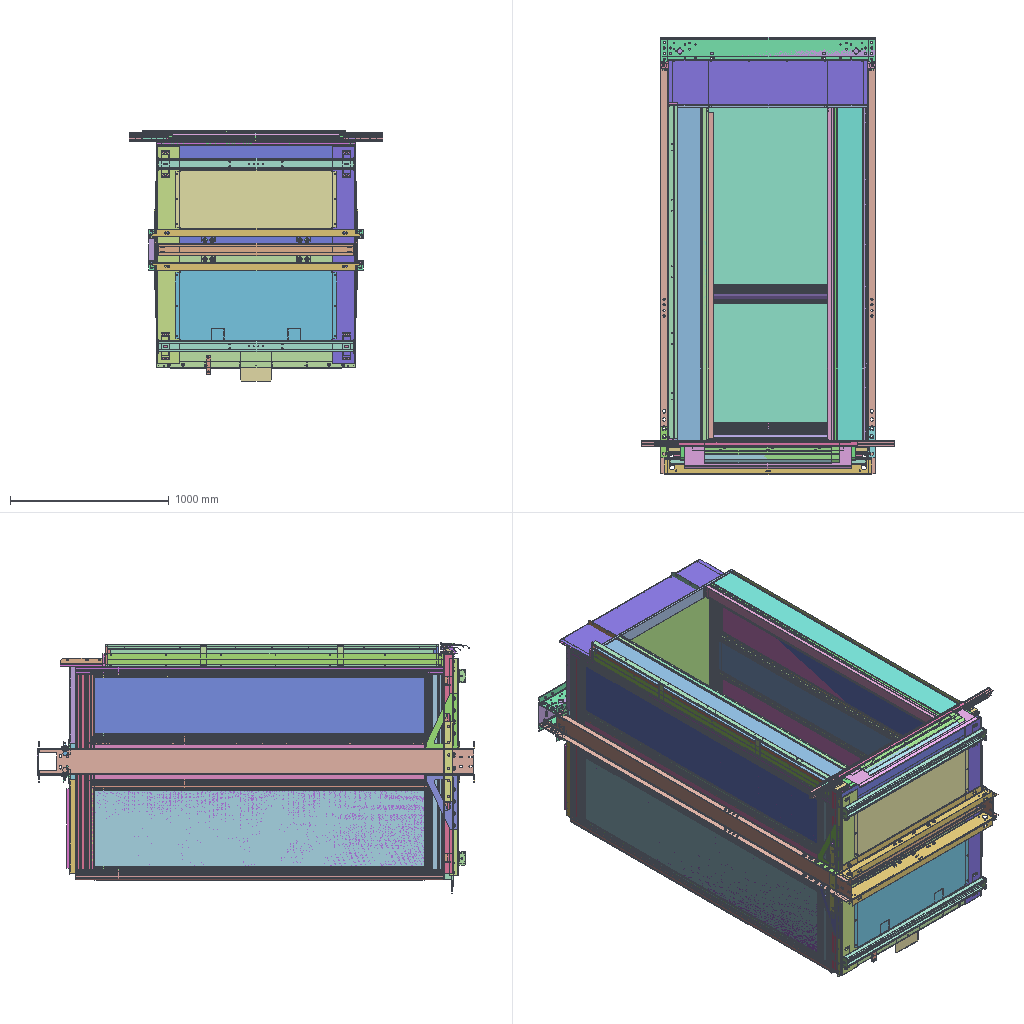Assembly | SolidWorks | 226 different items | 382 placed | box 1600 x 2756 x 1580 mm
Parts list (item | name | quantity | parent item | size | volume | features):
1 | (subassembly) | x1 | in 56 | 1250 x 2151 x 320 mm | 8404341 mm3 | features ReferencePattern 11, MirrorCompFeat 3
2 | (subassembly) | x1 | in 1 | 36 x 2116 x 253 mm | 1667556 mm3 | features ReferencePattern 7, MirrorCompFeat 2
3 | (subassembly) | x1 | in 1 | 36 x 2116 x 253 mm | 1688064 mm3 | features ReferencePattern 8, MirrorCompFeat 3
4 | (subassembly) | x1 | in 50 | 1354 x 89.5 x 1345 mm | 7454368 mm3 | features ReferencePattern 8, MirrorCompFeat 5
5 | (subassembly) | x1 | in 4 | 1250 x 1345 x 59.5 mm | 5102202 mm3 | features ReferencePattern 5, MirrorCompFeat 4, LocalLPattern 1
6 | (subassembly) | x1 | in 7 | 1250 x 70 x 1510 mm | 9091467 mm3 | features ReferencePattern 33, LocalLPattern 6, MirrorCompFeat 5
7 | (subassembly) | x1 | in 50 | 1250 x 70 x 1510 mm | 9091467 mm3 | -
8 | (subassembly) | x1 | in 50 | 1280 x 70 x 1465 mm | 13190412 mm3 | -
9 | (subassembly) | x1 | in 8 | 1280 x 70 x 1465 mm | 11467233 mm3 | features ReferencePattern 25, MirrorCompFeat 7, LocalLPattern 2
10 | (subassembly) | x1 | in 50 | 1250 x 299.8 x 80.3 mm | 1285406 mm3 | -
11 | (subassembly) | x1 | in 22 | 1350 x 2756 x 860 mm | 17468033 mm3 | features ReferencePattern 10, MirrorCompFeat 7, LocalLPattern 1
12 | (subassembly) | x1 | in 10 | 1250 x 299.5 x 80 mm | 853171 mm3 | features MirrorCompFeat 2, ReferencePattern 2
13 | (subassembly) | x1 | in 14 | 250 x 2116 x 80 mm | 1096241 mm3 | features MirrorCompFeat 1, ReferencePattern 1
14 | (subassembly) | x1 | in 50 | 282.3 x 2116 x 80 mm | 2341732 mm3 | -
15 | (subassembly) | x1 | in 16 | 250 x 2116 x 80 mm | 1147542 mm3 | features MirrorCompFeat 1, ReferencePattern 1
16 | (subassembly) | x1 | in 50 | 251 x 2116 x 80 mm | 2427688 mm3 | -
17 | (subassembly) | x1 | in 4 | 132 x 50 x 101 mm | 90791 mm3 | -
18 | (subassembly) | x1 | in 4 | 132 x 50 x 101 mm | 90791 mm3 | -
19 | (subassembly) | x1 | in 4 | 132 x 50 x 101 mm | 90791 mm3 | -
20 | (subassembly) | x1 | in 4 | 132 x 50 x 101 mm | 90791 mm3 | -
21 | (subassembly) | x1 | in 51 | 1600 x 178.321 x 70 mm | 4811022 mm3 | -
22 | (subassembly) | x1 | - | 1350 x 2756 x 1370 mm | 24130984 mm3 | features ReferencePattern 4, MirrorCompFeat 2
23 | (subassembly) | x1 | in 24 | 1050 x 60 x 37 mm | 345223 mm3 | features ReferencePattern 5, LocalLPattern 1, MirrorCompFeat 1
24 | (subassembly) | x1 | in 21 | 1520 x 122.321 x 40 mm | 769307 mm3 | features InContextFeatHolder 2
25 | (subassembly) | x1 | in 26 | 50 x 70 x 950 mm | 418927 mm3 | features ReferencePattern 3, LocalLPattern 1, MirrorCompFeat 1
26 | (subassembly) | x1 | in 21 | 60 x 178.321 x 1600 mm | 1702820 mm3 | -
27 | (subassembly) | x1 | in 28 | 60 x 70 x 800 mm | 384699 mm3 | features ReferencePattern 2, MirrorCompFeat 1
28 | (subassembly) | x1 | in 21 | 70 x 143.651 x 1130 mm | 1286253 mm3 | -
29 | (subassembly) | x1 | in 30 | 60 x 70 x 850 mm | 408712 mm3 | features ReferencePattern 2, MirrorCompFeat 1
30 | (subassembly) | x1 | in 21 | 1235 x 141.151 x 70 mm | 1052643 mm3 | -
31 | (subassembly) | x1 | in 35 | 1140 x 1260 x 70.147 mm | 18590168 mm3 | -
32 | (subassembly) | x1 | in 31 | 40 x 1260 x 1140 mm | 17028562 mm3 | -
33 | (subassembly) | x1 | in 22 | 1250 x 105 x 1370 mm | 4883387 mm3 | features ReferencePattern 8, MirrorCompFeat 2
34 | (subassembly) | x1 | in 31 | 1140 x 1260 x 30.147 mm | 1561605 mm3 | -
35 | (subassembly) | x1 | in 51 | - | 187293162 mm3 | -
36 | (subassembly) | x1 | in 35 | 1140 x 1260 x 75 mm | 31682872 mm3 | -
37 | (subassembly) | x1 | in 36 | 1113 x 1233 x 48 mm | 830275 mm3 | -
38 | (subassembly) | x1 | in 35 | 1140 x 1260 x 70 mm | 25062721 mm3 | -
39 | (subassembly) | x1 | in 38 | 1139 x 1259 x 30.281 mm | 733332 mm3 | -
40 | (subassembly) | x1 | in 38 | 1139 x 1259 x 40 mm | 807129 mm3 | -
41 | (subassembly) | x1 | in 35 | 1140 x 1260 x 70 mm | 26807789 mm3 | -
42 | (subassembly) | x1 | in 41 | 1139 x 1259 x 40 mm | 1605167 mm3 | -
43 | (subassembly) | x1 | in 41 | 1139 x 1259 x 40 mm | 1680362 mm3 | -
44 | (subassembly) | x1 | in 33 | 145 x 60 x 1370 mm | 1610892 mm3 | -
45 | (subassembly) | x1 | in 35 | 1140 x 1260 x 80 mm | 7783744 mm3 | -
46 | (subassembly) | x1 | in 45 | 1140 x 1260 x 36 mm | 6158512 mm3 | -
47 | (subassembly) | x1 | in 45 | 1140 x 1260 x 44 mm | 1625232 mm3 | -
48 | (subassembly) | x1 | in 35 | 1140 x 1260 x 60.087 mm | 6458843 mm3 | -
49 | (subassembly) | x1 | in 48 | 1140 x 1260 x 25.087 mm | 1538829 mm3 | -
50 | (subassembly) | x1 | in 51 | - | 297784141 mm3 | -
51 | (subassembly) | x1 | - | - | - | -
52 | (subassembly) | x1 | in 53 | 58 x 2100 x 140 mm | 731344 mm3 | features MirrorCompFeat 2, ReferencePattern 2
53 | (subassembly) | x1 | in 51 | 58 x 2132 x 140 mm | 854542 mm3 | -
54 | (subassembly) | x1 | in 33 | 145 x 60 x 1370 mm | 1610892 mm3 | -
55 | (subassembly) | x2 | in 56 | 56.572 x 22.358 x 2290 mm | 566961 mm3 | -
56 | (subassembly) | x1 | in 50 | - | 235752784 mm3 | features ReferencePattern 10, MirrorCompFeat 5
57 | - | x1 | in 11 | 350 x 45 x 200 mm | 201146 mm3 | features ICE 8, Fillet 3, FlatPattern 1, SMBaseFlange 1, SheetMetal 1
58 | - | x1 | in 16 | 17 x 30 x 2056 mm | 161613 mm3 | features Cut 1, EdgeFlange 1, FlatPattern 1, ICE 1, SMBaseFlange 1, SheetMetal 1
59 | - | x1 | in 16 | 209 x 34 x 2116 mm | 510788 mm3 | features ICE 2, FlatPattern 1, SMBaseFlange 1, SheetMetal 1
60 | - | x1 | in 16 | 80 x 1 x 2116 mm | 168632 mm3 | features FlatPattern 1, ICE 1, MirrorPattern 1, SMBaseFlange 1, SheetMetal 1
61 | - | x1 | in 15 | 246 x 76 x 25 mm | 27497 mm3 | features MirrorStock 1
62 | - | x12 | in 56 | 104 x 104 x 17 mm | 9651 mm3 | features ICE 3, FlatPattern 1, SMBaseFlange 1, SheetMetal 1
63 | - | x4 | in 1 | 240 x 85 x 17 mm | 19751 mm3 | features ICE 3, FlatPattern 1, MirrorPattern 1, SMBaseFlange 1, SheetMetal 1
64 | - | x1 | in 17 | 131 x 50 x 101 mm | 48396 mm3 | features ICE 6, EdgeFlange 1, Fillet 1, FlatPattern 1, SMBaseFlange 1, SheetMetal 1
65 | - | x1 | in 4 | 30 x 2 x 120 mm | 6643 mm3 | features Fillet 1, FlatPattern 1, ICE 1, SMBaseFlange 1, SheetMetal 1
66 | - | x2 | in 17 | 38 x 38 x 50 mm | 20238 mm3 | features Chamfer 2, MoveCopyBody 2, Extrusion 1, ICE 1
67 | - | x1 | in 4 | 1250 x 1 x 1306 mm | 1467099 mm3 | features ICE 10, FlatPattern 2, SMBaseFlange 1, SheetMetal 1
68 | - | x1 | in 11 | 1350 x 170 x 120 mm | 2114515 mm3 | features ICE 2, Chamfer 1, FlatPattern 1, SMBaseFlange 1, SheetMetal 1
69 | - | x2 | in 4 | 483.5 x 34 x 12 mm | 23557 mm3 | features SMBaseFlange 2, Chamfer 1, Cut 1, EdgeFlange 1, FlatPattern 1, ICE 1, MirrorPattern 1, SheetMetal 1
70 | - | x2 | in 4 | 590 x 34 x 12 mm | 29992 mm3 | features SMBaseFlange 2, Chamfer 1, Cut 1, EdgeFlange 1, FlatPattern 1, ICE 1, MirrorPattern 1, SheetMetal 1
71 | - | x1 | in 18 | 131 x 50 x 101 mm | 48396 mm3 | features MirrorStock 1
72 | - | x1 | in 19 | 131 x 50 x 101 mm | 48396 mm3 | features MirrorStock 1
73 | - | x2 | in 18 | 38 x 38 x 50 mm | 20238 mm3 | features MirrorStock 1
74 | - | x2 | in 19 | 38 x 38 x 50 mm | 20238 mm3 | features MirrorStock 1
75 | - | x1 | in 20 | 131 x 50 x 101 mm | 48396 mm3 | features MirrorStock 1
76 | - | x2 | in 20 | 38 x 38 x 50 mm | 20238 mm3 | features MirrorStock 1
77 | - | x1 | in 23 | 37 x 60 x 1050 mm | 331468 mm3 | features Cut 2, ICE 2, FlatPattern 1, SMBaseFlange 1, SheetMetal 1
78 | - | x6 | in 23 | 30.5 x 48 x 2 mm | 2292 mm3 | features Extrusion 1
79 | - | x4 | in 33 | 85 x 45 x 6 mm | 22107 mm3 | features Extrusion 1
80 | - | x1 | in 24 | 17 x 118.321 x 1100 mm | 138591 mm3 | features FlatPattern 1, ICE 1, SMBaseFlange 1, SheetMetal 1
81 | - | x1 | in 24 | 40 x 29.5 x 1520 mm | 285493 mm3 | features Emboss 1, Extrusion 1, ICE 1
82 | - | x1 | in 26 | 17 x 138.321 x 1050 mm | 153799 mm3 | features FlatPattern 1, ICE 1, SMBaseFlange 1, SheetMetal 1
83 | - | x1 | in 25 | 50 x 70 x 950 mm | 401871 mm3 | features ICE 3, FlatPattern 1, SMBaseFlange 1, SheetMetal 1
84 | - | x4 | in 25 | 43.5 x 60 x 2 mm | 4264 mm3 | features Chamfer 1, Extrusion 1
85 | - | x1 | in 26 | 60 x 40 x 1600 mm | 1130094 mm3 | features Emboss 1, Extrusion 1, ICE 1
86 | - | x1 | in 27 | 60 x 70 x 800 mm | 363963 mm3 | features ICE 3, FlatPattern 1, SMBaseFlange 1, SheetMetal 1
87 | - | x4 | in 27 | 53.5 x 60 x 2 mm | 5184 mm3 | features Chamfer 1, Extrusion 1
88 | - | x1 | in 28 | 70 x 35 x 1130 mm | 809219 mm3 | features Cut 1, Extrusion 1, ICE 1
89 | - | x1 | in 28 | 23.5 x 102.651 x 800 mm | 92335 mm3 | features FlatPattern 1, ICE 1, SMBaseFlange 1, SheetMetal 1
90 | - | x1 | in 33 | 1228 x 80 x 30 mm | 774609 mm3 | features EdgeFlange 2, ICE 2, FlatPattern 1, SMBaseFlange 1, SheetMetal 1
91 | - | x2 | in 30 | 23.5 x 102.651 x 850 mm | 98121 mm3 | features FlatPattern 1, ICE 1, SMBaseFlange 1, SheetMetal 1
92 | - | x1 | in 29 | 60 x 70 x 850 mm | 387976 mm3 | features ICE 3, FlatPattern 1, SMBaseFlange 1, SheetMetal 1
93 | - | x4 | in 29 | 53.5 x 60 x 2 mm | 5184 mm3 | features Chamfer 1, Extrusion 1
94 | - | x1 | in 30 | 70 x 29.5 x 1235 mm | 447688 mm3 | features Emboss 1, Extrusion 1, ICE 1
95 | - | x1 | in 32 | 1135 x 1255 x 5 mm | 7122125 mm3 | features Extrusion 1
96 | - | x1 | in 32 | 1140 x 1260 x 40 mm | 435262 mm3 | features Sweep 1
97 | - | x1 | in 32 | 1135 x 1255 x 6 mm | 8546550 mm3 | features Extrusion 1
98 | - | x2 | in 32 | 20 x 20 x 1215 mm | 239025 mm3 | features Extrusion 1
99 | - | x2 | in 32 | 20 x 20 x 1135 mm | 223287 mm3 | features Extrusion 1
100 | - | x1 | in 34 | 1140 x 1260 x 30 mm | 1498692 mm3 | features ICE 3, EdgeFlange 2, FlatPattern 1, SMBaseFlange 1, SheetMetal 1
101 | - | x1 | - | 1046 x 260 x 25 mm | 1454749 mm3 | features ICE 6, Fillet 1, FlatPattern 1, SMBaseFlange 1, SheetMetal 1
102 | - | x1 | in 34 | 151 x 20 x 399 mm | 62913 mm3 | features EdgeFlange 1, FlatPattern 1, MirrorPattern 1, SMBaseFlange 1, SheetMetal 1
103 | - | x1 | in 35 | 1140 x 1260 x 50 mm | 70907025 mm3 | features ICE 2, Extrusion 1
104 | - | x1 | in 37 | 1113 x 1233 x 48 mm | 780188 mm3 | features ICE 7, EdgeFlange 2, FlatPattern 1, SMBaseFlange 1, SheetMetal 1
105 | - | x1 | in 37 | 349.001 x 131.5 x 33.5 mm | 50088 mm3 | features EdgeFlange 1, FlatPattern 1, MirrorPattern 1, SMBaseFlange 1, SheetMetal 1
106 | - | x1 | in 36 | 1140 x 1260 x 27 mm | 30852596 mm3 | features ICE 1, WeldMemberFeat 1, WeldmentFeature 1
107 | - | x1 | in 39 | 1139 x 1259 x 30 mm | 692290 mm3 | features ICE 7, EdgeFlange 2, FlatPattern 1, SMBaseFlange 1, SheetMetal 1
108 | - | x1 | in 39 | 299 x 128.5 x 22 mm | 41042 mm3 | features EdgeFlange 1, FlatPattern 1, MirrorPattern 1, SMBaseFlange 1, SheetMetal 1
109 | - | x1 | in 38 | 1140 x 1260 x 30 mm | 23522260 mm3 | features ICE 1, WeldMemberFeat 1, WeldmentFeature 1
110 | - | x1 | in 40 | 1139 x 1259 x 40 mm | 764574 mm3 | features ICE 8, EdgeFlange 2, FlatPattern 1, SMBaseFlange 1, SheetMetal 1
111 | - | x1 | in 40 | 299 x 130.5 x 31 mm | 42555 mm3 | features Cut 1, EdgeFlange 1, FlatPattern 1, MirrorPattern 1, SMBaseFlange 1, SheetMetal 1
112 | - | x1 | - | 5 x 19 x 247 mm | 22965 mm3 | features 3DProfileFeature 1, Chamfer 1, Extrusion 1
113 | - | x1 | in 42 | 1139 x 1259 x 40 mm | 1562312 mm3 | features ICE 4, EdgeFlange 2, Cut 1, FlatPattern 1, SMBaseFlange 1, SheetMetal 1
114 | - | x1 | in 42 | 299 x 130.5 x 31 mm | 42855 mm3 | features EdgeFlange 1, FlatPattern 1, MirrorPattern 1, SMBaseFlange 1, SheetMetal 1
115 | - | x1 | in 41 | 1140 x 1260 x 30 mm | 23522260 mm3 | features ICE 1, WeldMemberFeat 1, WeldmentFeature 1
116 | - | x1 | in 43 | 1139 x 1259 x 40 mm | 1637806 mm3 | features ICE 5, EdgeFlange 2, Cut 1, FlatPattern 1, SMBaseFlange 1, SheetMetal 1
117 | - | x1 | in 43 | 299 x 130.5 x 31 mm | 42555 mm3 | features Cut 1, EdgeFlange 1, FlatPattern 1, MirrorPattern 1, SMBaseFlange 1, SheetMetal 1
118 | - | x1 | in 46 | 1140 x 1260 x 1 mm | 1435171 mm3 | features Cut 2, Extrusion 1
119 | - | x1 | in 46 | 1135 x 1255 x 3 mm | 4273275 mm3 | features Extrusion 1
120 | - | x1 | in 47 | 137.5 x 33 x 299 mm | 45429 mm3 | features EdgeFlange 1, FlatPattern 1, MirrorPattern 1, SMBaseFlange 1, SheetMetal 1
121 | - | x1 | in 46 | 1140 x 1260 x 35 mm | 450066 mm3 | features WeldMemberFeat 1, WeldmentFeature 1
122 | - | x1 | in 47 | 1140 x 1260 x 44 mm | 1579803 mm3 | features ICE 4, EdgeFlange 2, Cut 1, FlatPattern 1, SMBaseFlange 1, SheetMetal 1
123 | - | x2 | in 33 | 40 x 1228 x 70 mm | 399285 mm3 | features FlatPattern 1, ICE 1, SMBaseFlange 1, SheetMetal 1
124 | - | x1 | in 49 | 1140 x 1260 x 25 mm | 1476577 mm3 | features ICE 4, EdgeFlange 2, FlatPattern 1, SMBaseFlange 1, SheetMetal 1
125 | - | x1 | in 49 | 150.5 x 17 x 399 mm | 62251 mm3 | features EdgeFlange 1, FlatPattern 1, MirrorPattern 1, SMBaseFlange 1, SheetMetal 1
126 | - | x1 | in 48 | 1260 x 1140 x 35 mm | 4920014 mm3 | features ICE 1, WeldMemberFeat 1, WeldmentFeature 1
127 | - | x1 | in 51 | 225 x 80 x 2116 mm | 3306402 mm3 | features Fillet 6, ICE 5, Extrusion 1, MirrorSolid 1
128 | - | x1 | in 51 | 240 x 80 x 2116 mm | 3439932 mm3 | features Fillet 6, ICE 5, Extrusion 1, MirrorSolid 1
129 | - | x1 | in 50 | 1198 x 1399 x 16 mm | 26240288 mm3 | features Chamfer 1, Extrusion 1
130 | - | x1 | in 51 | 70 x 15 x 750 mm | 474672 mm3 | features ICE 14, Fillet 3, Extrusion 1, MirrorSolid 1
131 | - | x1 | in 52 | 58 x 140 x 2100 mm | 680862 mm3 | features ICE 3, FlatPattern 1, MirrorPattern 1, SMBaseFlange 1, SheetMetal 1
132 | - | x2 | in 52 | 125 x 40 x 2 mm | 10000 mm3 | features Extrusion 1
133 | - | x2 | in 53 | 56 x 80 x 16 mm | 61599 mm3 | features Extrusion 1, ICE 1
134 | - | x1 | - | 30 x 500 x 50 mm | 112732 mm3 | features ICE 2, FlatPattern 1, SMBaseFlange 1, SheetMetal 1
135 | - | x1 | in 52 | 55 x 136 x 30 mm | 15241 mm3 | features Cut 4, EdgeFlange 2, FlatPattern 1, SMBaseFlange 1, SheetMetal 1
136 | - | x1 | in 52 | 55 x 136 x 30 mm | 15241 mm3 | features MirrorStock 1
137 | - | x1 | - | 30 x 557 x 50 mm | 125994 mm3 | features ICE 2, FlatPattern 1, SMBaseFlange 1, SheetMetal 1
138 | - | x1 | in 44 | 145 x 60 x 1370 mm | 1590981 mm3 | features ICE 3, Cut 1, EdgeFlange 1, FlatPattern 1, SMBaseFlange 1, SheetMetal 1
139 | - | x1 | in 22 | 1020 x 441 x 10 mm | 461945 mm3 | features ICE 4, SMBaseFlange 2, Cut 1, EdgeFlange 1, Fillet 1, FlatPattern 1, SheetMetal 1
140 | - | x1 | in 54 | 145 x 60 x 1370 mm | 1590981 mm3 | features MirrorStock 1
141 | - | x1 | in 11 | 350 x 45 x 200 mm | 201146 mm3 | features MirrorStock 1
142 | - | x1 | in 11 | 350 x 45 x 200 mm | 201146 mm3 | features MirrorStock 1
143 | - | x1 | in 11 | 350 x 45 x 200 mm | 201146 mm3 | features MirrorStock 1
144 | - | x1 | in 51 | 12 x 73 x 1250 mm | 455000 mm3 | features Extrusion 1
145 | - | x2 | in 56 | 410 x 2136 x 18 mm | 8644224 mm3 | features ICE 2, WeldMemberFeat 1, WeldmentFeature 1
146 | - | x2 | in 56 | 540 x 2136 x 18 mm | 11415432 mm3 | features ICE 2, WeldMemberFeat 1, WeldmentFeature 1
147 | - | x1 | in 56 | 1250 x 2136 x 18 mm | 26549237 mm3 | features ICE 3, MirrorPattern 1, WeldMemberFeat 1, WeldmentFeature 1
148 | - | x1 | in 56 | 1140 x 2136 x 18 mm | 43830720 mm3 | features ICE 2, WeldMemberFeat 1, WeldmentFeature 1
149 | - | x2 | in 55 | 56.572 x 22.358 x 2285 mm | 383048 mm3 | features Extrusion 1
150 | - | x1 | in 22 | 1020 x 371 x 10 mm | 392822 mm3 | features ICE 3, Cut 1, EdgeFlange 1, Fillet 1, FlatPattern 1, SMBaseFlange 1, SheetMetal 1
151 | - | x2 | in 55 | 46.782 x 13.535 x 2290 mm | 183913 mm3 | features Extrusion 1
152 | - | x1 | in 56 | 1140 x 2136 x 62.186 mm | 24296668 mm3 | features ICE 7, MirrorSolid 1, WeldMemberFeat 1, WeldmentFeature 1
153 | - | x1 | in 56 | 1250 x 2316 x 1345 mm | 13061809 mm3 | features WeldMemberFeat 5, ICE 4, 3DProfileFeature 1, WeldmentFeature 1
154 | - | x4 | in 1 | 25 x 50 x 2116 mm | 659198 mm3 | features Extrusion 1
155 | - | x4 | in 1 | 14.605 x 34.798 x 2116 mm | 344207 mm3 | features Extrusion 1
156 | - | x4 | in 1 | 9.4 x 46.998 x 2116 mm | 239025 mm3 | features Extrusion 1
157 | - | x1 | in 2 | 240 x 2116 x 23 mm | 875220 mm3 | features Chamfer 2, ICE 2, Cut 1, FlatPattern 1, SMBaseFlange 1, SheetMetal 1
158 | - | x1 | in 2 | 235 x 2116 x 33 mm | 746266 mm3 | features ICE 4, Chamfer 2, Fillet 1, FlatPattern 1, SMBaseFlange 1, SheetMetal 1
159 | - | x1 | in 3 | 20 x 30 x 300 mm | 20507 mm3 | features Cut 1, Fillet 1, FlatPattern 1, SMBaseFlange 1, SheetMetal 1
160 | - | x1 | in 3 | 240 x 2116 x 23 mm | 875220 mm3 | features Chamfer 2, ICE 2, Cut 1, FlatPattern 1, SMBaseFlange 1, SheetMetal 1
161 | - | x3 | in 11 | 160 x 50 x 1350 mm | 1636068 mm3 | features ICE 4, FlatPattern 1, SMBaseFlange 1, SheetMetal 1
162 | - | x1 | in 3 | 235 x 2116 x 33 mm | 746266 mm3 | features ICE 4, Chamfer 2, Fillet 1, FlatPattern 1, SMBaseFlange 1, SheetMetal 1
163 | - | x24 | in 2, 3 | 12 x 12 x 16.74 mm | 900.506 mm3 | features ICE 2, Extrusion 1, MoveCopyBody 1
164 | - | x4 | in 2, 3 | 10 x 30 x 232 mm | 17632 mm3 | features ExtruThin 1
165 | - | x1 | in 56 | 1140 x 2136 x 71.386 mm | 51691729 mm3 | features ICE 13, MirrorSolid 3, LPattern 1, WeldMemberFeat 1, WeldmentFeature 1
166 | - | x1 | in 56 | 1250 x 2136 x 18 mm | 26549237 mm3 | features MirrorStock 1
167 | - | x1 | in 4 | 120 x 42 x 120 mm | 202989 mm3 | features Extrusion 1, ICE 1
168 | - | x4 | in 4 | 115 x 90 x 15 mm | 51294 mm3 | features ICE 2, FlatPattern 1, SMBaseFlange 1, SheetMetal 1
169 | - | x2 | in 5 | 1169 x 38 x 80 mm | 279454 mm3 | features FlatPattern 1, ICE 1, SMBaseFlange 1, SheetMetal 1
170 | - | x2 | in 5 | 48 x 20 x 500 mm | 108566 mm3 | features FlatPattern 1, SMBaseFlange 1, SheetMetal 1
171 | - | x2 | in 11 | 1310 x 100 x 50 mm | 1180927 mm3 | features ICE 4, FlatPattern 1, MirrorPattern 1, SMBaseFlange 1, SheetMetal 1
172 | - | x2 | in 5 | 700 x 38 x 80 mm | 166325 mm3 | features FlatPattern 1, ICE 1, SMBaseFlange 1, SheetMetal 1
173 | - | x1 | in 5 | 1250 x 1345 x 39.5 mm | 2576093 mm3 | features Cut 6, ICE 4, EdgeFlange 2, Fillet 1, FlatPattern 1, SMBaseFlange 1, SheetMetal 1
174 | - | x1 | in 5 | 60 x 38 x 1250 mm | 171739 mm3 | features ICE 3, Cut 2, SMBaseFlange 2, Chamfer 1, Fillet 1, FlatPattern 1, SheetMetal 1
175 | - | x1 | in 5 | 1302 x 38 x 40 mm | 208795 mm3 | features Cut 4, ICE 2, SMBaseFlange 2, FlatPattern 1, SheetMetal 1
176 | - | x2 | in 5 | 300 x 36 x 40 mm | 55080 mm3 | features Cut 2, EdgeFlange 1, FlatPattern 1, SMBaseFlange 1, SheetMetal 1
177 | - | x2 | in 5 | 1169 x 38 x 46 mm | 238296 mm3 | features Cut 1, FlatPattern 1, ICE 1, SMBaseFlange 1, SheetMetal 1
178 | - | x1 | in 5 | 1169 x 38 x 46 mm | 238296 mm3 | features Cut 1, FlatPattern 1, ICE 1, SMBaseFlange 1, SheetMetal 1
179 | - | x1 | in 5 | 1302 x 38 x 40 mm | 208795 mm3 | features MirrorStock 1
180 | - | x1 | in 6 | 200 x 200 x 3 mm | 119400 mm3 | features Chamfer 1, Extrusion 1
181 | - | x1 | in 6 | 120 x 30 x 2 mm | 6777 mm3 | features Extrusion 1, Fillet 1, ICE 1
182 | - | x22 | in 6 | 73 x 43 x 3 mm | 7278 mm3 | features Chamfer 1, FlatPattern 1, ICE 1, SMBaseFlange 1, SheetMetal 1
183 | - | x6 | in 6 | 26 x 43 x 3 mm | 3279 mm3 | features Chamfer 1, Extrusion 1
184 | - | x1 | in 6 | 77 x 50 x 1420 mm | 692252 mm3 | features ICE 4, Cut 1, Fillet 1, FlatPattern 1, SMBaseFlange 1, SheetMetal 1
185 | - | x1 | in 6 | 1425 x 70 x 1250 mm | 5618902 mm3 | features ICE 10, Cut 3, Fillet 1, FlatPattern 1, SMBaseFlange 1, SheetMetal 1
186 | - | x7 | in 6 | 25 x 1095 x 50 mm | 206464 mm3 | features FlatPattern 1, ICE 1, SMBaseFlange 1, SheetMetal 1
187 | - | x1 | in 6 | 30 x 50 x 1095 mm | 331528 mm3 | features Cut 1, FlatPattern 1, ICE 1, SMBaseFlange 1, SheetMetal 1
188 | - | x1 | in 6 | 77 x 50 x 1420 mm | 692252 mm3 | features MirrorStock 1
189 | - | x1 | in 9 | 120 x 30 x 2 mm | 6777 mm3 | features Extrusion 1, Fillet 1, ICE 1
190 | - | x8 | in 9 | 26 x 53 x 3 mm | 4059 mm3 | features Chamfer 1, FlatPattern 1, SMBaseFlange 1, SheetMetal 1
191 | - | x8 | in 9 | 30 x 53 x 3 mm | 4695 mm3 | features Chamfer 1, FlatPattern 1, SMBaseFlange 1, SheetMetal 1
192 | - | x1 | in 11 | 405 x 88.5 x 88 mm | 988805 mm3 | features ICE 3, Fillet 1, Revolution 1
193 | - | x6 | in 9 | 36 x 55 x 3 mm | 5865 mm3 | features Chamfer 1, Extrusion 1
194 | - | x1 | in 9 | 70 x 62 x 1380 mm | 672771 mm3 | features ICE 10, SMBaseFlange 5, Cut 1, FlatPattern 1, SheetMetal 1
195 | - | x2 | in 9 | 40 x 1240 x 62 mm | 630088 mm3 | features SMBaseFlange 2, Cut 1, Fillet 1, FlatPattern 1, SheetMetal 1
196 | - | x4 | in 9 | 25 x 1249 x 62 mm | 374837 mm3 | features SMBaseFlange 2, Cut 1, Fillet 1, FlatPattern 1, ICE 1, SheetMetal 1
197 | - | x1 | in 9 | 1425 x 70 x 1260 mm | 5663138 mm3 | features ICE 10, Cut 1, Fillet 1, FlatPattern 1, SMBaseFlange 1, SheetMetal 1
198 | - | x2 | in 9 | 500 x 49 x 4 mm | 94037 mm3 | features FlatPattern 1, ICE 1, MirrorPattern 1, SMBaseFlange 1, SheetMetal 1
199 | - | x2 | in 9 | 500 x 52 x 10 mm | 250092 mm3 | features FlatPattern 1, ICE 1, MirrorPattern 1, SMBaseFlange 1, SheetMetal 1
200 | - | x1 | in 9 | 40 x 62 x 1260 mm | 502102 mm3 | features ICE 2, Cut 1, Fillet 1, FlatPattern 1, SMBaseFlange 1, SheetMetal 1
201 | - | x2 | in 9 | 62 x 200 x 122 mm | 183661 mm3 | features EdgeFlange 1, FlatPattern 1, ICE 1, SMBaseFlange 1, SheetMetal 1
202 | - | x1 | in 8 | 1260 x 1400 x 1 mm | 1723179 mm3 | features ICE 4, FlatPattern 2, Cut 1, Fillet 1, MirrorPattern 1, SMBaseFlange 1, SheetMetal 1
203 | - | x4 | in 22 | 170 x 52 x 38 mm | 231199 mm3 | features ICE 2, Extrusion 1, MirrorPattern 1, RefAxis 1
204 | - | x1 | in 9 | 70 x 62 x 1380 mm | 672771 mm3 | features MirrorStock 1
205 | - | x1 | in 12 | 80 x 299.5 x 1250 mm | 750751 mm3 | features ICE 11, Cut 6, EdgeFlange 5, SMBaseFlange 4, Chamfer 1, FlatPattern 1, LPattern 1, SheetMetal 1
206 | - | x1 | in 12 | 296 x 25 x 76.7 mm | 12498 mm3 | features Cut 2, EdgeFlange 2, FlatPattern 1, ICE 1, LPattern 1, SMBaseFlange 1, SheetMetal 1
207 | - | x1 | in 12 | 298 x 15 x 78.5 mm | 38712 mm3 | features ICE 3, Cut 2, EdgeFlange 2, FlatPattern 1, SMBaseFlange 1, SheetMetal 1
208 | - | x1 | in 10 | 283.5 x 64 x 1250 mm | 432234 mm3 | features ICE 2, FlatPattern 1, SMBaseFlange 1, SheetMetal 1
209 | - | x1 | in 12 | 296 x 25 x 76.7 mm | 12498 mm3 | features MirrorStock 1
210 | - | x1 | in 12 | 298 x 15 x 78.5 mm | 38712 mm3 | features MirrorStock 1
211 | - | x1 | in 13 | 246 x 76 x 25 mm | 25378 mm3 | features ICE 5, EdgeFlange 3, Cut 2, FlatPattern 1, SMBaseFlange 1, SheetMetal 1
212 | - | x1 | in 13 | 250 x 80 x 2116 mm | 1045484 mm3 | features ICE 6, Cut 4, EdgeFlange 2, MirrorPattern 2, Fillet 1, FlatPattern 1, SMBaseFlange 1, SheetMetal 1
213 | - | x2 | in 11 | 160 x 45 x 2739 mm | 3145036 mm3 | features ICE 3, Cut 1, Fillet 1, FlatPattern 1, SMBaseFlange 1, SheetMetal 1
214 | - | x1 | in 14 | 98.4 x 25 x 2051 mm | 201768 mm3 | features ICE 2, EdgeFlange 1, FlatPattern 1, SMBaseFlange 1, SheetMetal 1
215 | - | x1 | in 14 | 35 x 35 x 2056 mm | 202689 mm3 | features FlatPattern 1, ICE 1, MirrorPattern 1, SMBaseFlange 1, SheetMetal 1
216 | - | x1 | in 14 | 17 x 30 x 2056 mm | 161613 mm3 | features Cut 1, EdgeFlange 1, FlatPattern 1, ICE 1, SMBaseFlange 1, SheetMetal 1
217 | - | x1 | in 14 | 209 x 34 x 2116 mm | 510788 mm3 | features ICE 2, FlatPattern 1, SMBaseFlange 1, SheetMetal 1
218 | - | x1 | in 14 | 80 x 1 x 2116 mm | 168632 mm3 | features FlatPattern 1, ICE 1, MirrorPattern 1, SMBaseFlange 1, SheetMetal 1
219 | - | x1 | in 13 | 246 x 76 x 25 mm | 25378 mm3 | features MirrorStock 1
220 | - | x1 | in 15 | 246 x 76 x 25 mm | 27497 mm3 | features ICE 6, EdgeFlange 3, Cut 1, FlatPattern 1, SMBaseFlange 1, SheetMetal 1
221 | - | x1 | in 15 | 250 x 80 x 2116 mm | 1092548 mm3 | features ICE 5, Cut 3, EdgeFlange 2, Fillet 1, FlatPattern 1, MirrorPattern 1, SMBaseFlange 1, SheetMetal 1
222 | - | x1 | in 16 | 98.4 x 25 x 2051 mm | 236423 mm3 | features Cut 1, EdgeFlange 1, FlatPattern 1, ICE 1, SMBaseFlange 1, SheetMetal 1
223 | - | x1 | in 16 | 35 x 35 x 2056 mm | 202689 mm3 | features FlatPattern 1, ICE 1, MirrorPattern 1, SMBaseFlange 1, SheetMetal 1
224 | hex nuts, style 1-grades ab gb | x1 | - | - | - | -
225 | hexagon weld nuts gb | x1 | - | - | - | -
226 | plain washers--product grade c gb | x1 | - | - | - | -
Mates (type | each side: item.copy, entity, surface, feature), first 459 of 711 lines:
In the top assembly
Coincident | 51.1 plane | 22.1 plane | 2 times
Coincident | 188.1 face plane | 203.1 face plane  Mirror 1
In subassembly 22
Coincident | 22.2 face | 22.2 face
Concentric | 22.2 face | 22.2 face
Coincident | 11.1 plane | 22.2 plane | 3 times
Coincident | 33.1 plane | 22.2 plane | 2 times
DistanceDim | 213.1 face plane  Base - Flange 1 | 138.1 face plane  Base - Flange 1
Concentric | 138.1 axis | assembly face | 2 times
Coincident | 138.1 face plane  Base - Flange 1 | assembly face | 2 times
Coincident | 138.1 face plane  Base - Flange 1 | 203.2 face plane  Mirror 1
Coincident | 138.1 axis | 203.2 axis | 2 times
Coincident | 138.1 face plane  Base - Flange 1 | 203.3 face plane  Mirror 1
Coincident | 138.1 axis | 203.3 axis | 2 times
Coincident | 140.1 face plane 26-4047 Bracket Edge Beam _ Mirror  | 139.1 face plane  Base - Flange 1
Coincident | 139.1 plane | 22.2 plane
Coincident | 140.1 face plane 26-4047 Bracket Edge Beam _ Mirror  | 150.1 face plane  Base - Flange 1
Coincident | 139.1 plane | 150.1 plane
DistanceDim | 123.1 face plane  Base - Flange 1 | 139.1 face plane  Edge - Flange 1
DistanceDim | 150.1 face plane  Edge - Flange 1 | 123.2 face plane  Base - Flange 1
In subassembly 11
Coincident | 11.2 face | 11.2 face
Concentric | 11.2 face | 11.2 face
Coincident | 161.1 plane | 11.2 plane
Coincident | 213.2 plane | 11.2 plane
Coincident | 161.1 face plane  Base - Flange 1 | 213.2 face plane  Base - Flange 1
Coincident | 213.2 face plane  Base - Flange 1 | 57.1 face plane  Base - Flange 1 | 2 times
Coincident | 68.1 plane | 11.2 plane | 3 times
DistanceDim | 68.1 face plane  Base - Flange 1 | 213.2 face plane  Base - Flange 1
Coincident | 213.2 face plane  Base - Flange 1 | 68.1 face plane  Base - Flange 1
DistanceDim | 57.1 face plane  Base - Flange 1 | 213.2 face plane  Base - Flange 1
Coincident | 171.1 plane | 11.2 plane
DistanceDim | 141.1 face plane | 171.1 face plane  Base - Flange 1
DistanceDim | 171.2 face cylinder  Cut - Extrude 1 | 171.1 face cylinder  Cut - Extrude 1
Concentric | 171.1 face cylinder  Cut - Extrude 4 | 192.1 face
DistanceDim | 192.1 face | 171.1 face plane  Base - Flange 1
Slot | 192.1 face | 171.1 face cylinder  Cut - Extrude 4
Coincident | assembly plane | 11.2 plane | 2 times
Coincident | 171.1 edge | assembly face
DistanceDim | 161.1 face plane  Base - Flange 1 | 213.2 face plane  Base - Flange 1
In subassembly 33
Coincident | 33.2 face | 33.2 face
Concentric | 33.2 face | 33.2 face
Coincident | 44.1 plane | 33.2 plane
Coincident | 138.2 face plane  Base - Flange 1 | 33.2 plane
Coincident | 123.3 plane | 33.2 plane
Coincident | 138.2 face plane  Base - Flange 1 | 123.3 face plane  Base - Flange 1
Coincident | 90.1 plane | 33.2 plane | 2 times
Coincident | 90.1 face plane  Base - Flange 1 | 138.2 face plane  Base - Flange 1
DistanceDim | 138.2 face plane  Base - Flange 1 | 140.2 face plane 26-4047 Bracket Edge Beam _ Mirror 
Coincident | assembly plane | 33.2 plane | 2 times
Coincident | 138.2 face plane  Base - Flange 1 | 33.2 face
DistanceDim | 123.3 face plane  Base - Flange 1 | 138.2 face plane  Base - Flange 1
Coincident | 123.3 face plane  Base - Flange 1 | 79.1 face plane  Boss - Extrude 1
Coincident | 123.3 edge | 79.1 face plane  Boss - Extrude 1
DistanceDim | 79.1 face plane  Boss - Extrude 1 | 123.3 face plane  Base - Flange 1
Coincident | 123.3 face plane  Base - Flange 1 | 79.2 face plane  Boss - Extrude 1
Coincident | 138.2 face plane  Base - Flange 1 | 79.2 face plane  Boss - Extrude 1
Coincident | 79.1 face plane  Boss - Extrude 1 | 79.2 face plane  Boss - Extrude 1
In subassembly 44
Coincident | 44.2 face | 44.2 face
Concentric | 44.2 face | 44.2 face
Coincident | 138.3 plane | 44.2 plane | 3 times
In subassembly 51
Coincident | 51.2 face | 51.2 face
Concentric | 51.2 face | 51.2 face
Coincident | 50.1 plane | 51.2 plane | 3 times
DistanceDim | 153.1 face plane 25 Profile 25 Profile Small Post (Latest) (1) | 77.1 face plane  Base - Flange 1
DistanceDim | 81.1 face plane  Boss - Extrude 1 | 153.1 face plane 25 Profile 25 Profile Small Post (Latest) (1)
Coincident | 153.1 plane | 21.1 plane
Coincident | 185.1 face plane  Base - Flange 1 | 128.1 face plane  Mirror 1
Coincident | 185.1 face plane  Base - Flange 1 | 127.1 face plane  Boss - Extrude 3
Coincident | 153.1 face plane 25 Profile 25 Profile Small Post (Latest) (1) | 127.1 face plane  Boss - Extrude 2
Coincident | 153.1 face plane 25 Profile 25 Profile Small Post (Latest) (1) | 130.1 face plane  Boss - Extrude 1 | 2 times
Coincident | 153.1 plane | 130.1 plane
Coincident | 81.1 face plane  Boss - Extrude 1 | 144.1 face plane  Boss - Extrude 1
Coincident | 77.1 face plane  Base - Flange 1 | 144.1 face plane  Boss - Extrude 1
Coincident | 144.1 plane | 51.2 plane
Coincident | 153.1 face plane 25 Profile 25 Profile Small Post (Latest) (1) | 131.1 face plane  Base - Flange 1
Coincident | 153.1 face plane 25 Profile 25 Profile Small Post (Latest) (1) | 128.1 face plane  Boss - Extrude 2
Coincident | 153.1 face plane 25 Profile 25 Profile Small Post (Latest) (1) | 128.1 face plane  Boss - Extrude 1
Coincident | 153.1 face plane 25 Car GC505&506(1) | 127.1 face plane  Boss - Extrude 1
DistanceDim | 103.1 face plane  Boss - Extrude 1 | 153.1 face plane 25 Car GC505&506(1) | 2 times
Coincident | 173.1 face plane  Base - Flange 1 | 103.1 face plane  Boss - Extrude 1
Coincident | 51.2 plane | 50.1 plane | 2 times
Coincident | 185.1 face plane  Base - Flange 1 | 51.2 face
In subassembly 35
Coincident | 35.1 face | 35.1 face
Concentric | 35.1 face | 35.1 face
Coincident | 103.2 plane | 35.1 plane | 2 times
Coincident | 103.2 face plane  Boss - Extrude 1 | 35.1 plane
Coincident | 103.2 face plane  Boss - Extrude 1 | 124.1 face plane  Base - Flange 1
Coincident | 48.1 plane | 35.1 plane | 2 times
Coincident | 36.1 plane | 35.1 plane | 2 times
Coincident | 103.2 face plane  Boss - Extrude 1 | 104.1 face plane  Base - Flange 1
Coincident | 103.2 face plane  Boss - Extrude 1 | 122.1 face plane  Base - Flange 1
Coincident | 45.1 plane | 35.1 plane | 2 times
Coincident | 41.1 plane | 35.1 plane | 2 times
Coincident | 103.2 face plane  Boss - Extrude 1 | 113.1 face plane  Base - Flange 1
Coincident | 38.1 plane | 35.1 plane | 2 times
Coincident | 103.2 face plane  Boss - Extrude 1 | 107.1 face plane  Base - Flange 1
Coincident | 32.1 plane | 35.1 plane
Coincident | 31.1 plane | 35.1 plane
Coincident | 124.1 face plane  Base - Flange 1 | 100.1 face plane  Base - Flange 1
In subassembly 45
Coincident | 45.2 face | 45.2 face
Concentric | 45.2 face | 45.2 face
Coincident | 47.1 plane | 45.2 plane | 2 times
Coincident | 46.1 plane | 45.2 plane | 2 times
Coincident | 118.1 face plane  Boss - Extrude 1 | 122.2 face plane  Edge - Flange 2
Coincident | 122.2 face plane  Base - Flange 1 | 45.2 plane
In subassembly 46
Coincident | 121.1 plane | 46.2 plane | 2 times
Coincident | 121.1 face plane  Backlit Panel Profile Frame (1) | 46.2 plane
Coincident | 119.1 plane | 46.2 plane | 2 times
Coincident | 119.1 face plane  Boss - Extrude 1 | 121.1 edge
Coincident | 121.1 face plane  Backlit Panel Profile Frame (1) | 118.2 face plane  Boss - Extrude 1
Coincident | 118.2 plane | 46.2 plane | 2 times
In subassembly 47
Coincident | 47.2 face | 47.2 face
Concentric | 47.2 face | 47.2 face
Coincident | 122.3 face plane  Base - Flange 1 | 47.2 plane
Coincident | 122.3 plane | 47.2 plane | 2 times
Coincident | 122.3 face plane  Base - Flange 1 | 120.1 edge
Coincident | 122.3 face plane  Front Fan  | 120.1 edge | 2 times
Width | 122.3 face plane  Front Fan  | 122.3 face plane  Front Fan  | 120.1 face plane  Edge - Flange 1 | 120.1 face plane  Mirror 1
Coincident | 122.3 face plane  Base - Flange 1 | 120.2 edge
Coincident | 122.3 face | 120.2 edge | 2 times
Width | 120.2 face | 120.2 face | 122.3 face | 122.3 face
In subassembly 38
Coincident | 38.2 face | 38.2 face
Concentric | 38.2 face | 38.2 face
Coincident | 39.1 plane | 38.2 plane | 2 times
Coincident | 107.2 face plane  Base - Flange 1 | 38.2 plane
Coincident | 109.1 plane | 38.2 plane | 2 times
Coincident | 109.1 face plane  Ceiling Profile Starry Ceiling Profile ( 250403 ) (1) | 107.2 face plane  Edge - Flange 2
Coincident | 40.1 plane | 38.2 plane | 2 times
Coincident | 109.1 face plane  Ceiling Profile Starry Ceiling Profile ( 250403 ) (1) | 110.1 face plane  Edge - Flange 2
In subassembly 39
Coincident | 39.2 face | 39.2 face
Concentric | 39.2 face | 39.2 face
Coincident | 107.3 plane | 39.2 plane | 2 times
Coincident | 107.3 face plane  Base - Flange 1 | 39.2 plane
Width | 108.1 face plane  Mirror 1 | 108.1 face plane  Edge - Flange 1 | 107.3 face plane  Front Fan  | 107.3 face plane  Front Fan 
Coincident | 107.3 face plane  Base - Flange 1 | 108.1 edge
Coincident | 107.3 face plane  Front Fan  | 108.1 edge | 2 times
Width | 108.2 face | 108.2 face | 107.3 face | 107.3 face
Coincident | 107.3 face plane  Base - Flange 1 | 108.2 edge
Coincident | 107.3 face | 108.2 edge | 2 times
In subassembly 40
Coincident | 40.2 face | 40.2 face
Concentric | 40.2 face | 40.2 face
Coincident | 110.2 plane | 40.2 plane | 2 times
Coincident | 110.2 face plane  Base - Flange 1 | 40.2 plane
Width | 111.1 face plane  Mirror 1 | 111.1 face plane  Edge - Flange 1 | 110.2 face plane  Front Fan  | 110.2 face plane  Front Fan 
Coincident | 110.2 face plane  Base - Flange 1 | 111.1 edge
Coincident | 110.2 face plane  Front Fan  | 111.1 edge | 2 times
Width | 111.2 face | 111.2 face | 110.2 face | 110.2 face
Coincident | 110.2 face plane  Base - Flange 1 | 111.2 edge
Coincident | 110.2 face | 111.2 edge | 2 times
In subassembly 48
Coincident | 48.2 face | 48.2 face
Concentric | 48.2 face | 48.2 face
Coincident | 49.1 plane | 48.2 plane | 2 times
Coincident | 124.2 face plane  Base - Flange 1 | 48.2 plane
Coincident | 126.1 plane | 48.2 plane | 2 times
Coincident | 124.2 face plane  Edge - Flange 2 | 126.1 face plane  Backlit Panel Profile Frame (1)
In subassembly 49
Coincident | 49.2 face | 49.2 face
Concentric | 49.2 face | 49.2 face
Coincident | 124.3 plane | 49.2 plane | 2 times
Coincident | 124.3 face plane  Base - Flange 1 | 49.2 plane
Coincident | 125.1 plane | 49.2 plane
Coincident | 124.3 face plane  Base - Flange 1 | 125.1 edge
Coincident | 124.3 face plane  Front Fan  | 125.1 edge | 2 times
Width | 125.2 face | 125.2 face | 124.3 face | 124.3 face
Coincident | 124.3 face | 125.2 edge | 2 times
Coincident | 124.3 face plane  Base - Flange 1 | 125.2 edge
In subassembly 31
Coincident | 31.2 face | 31.2 face
Concentric | 31.2 face | 31.2 face
Coincident | 32.2 plane | 31.2 plane | 2 times
Coincident | 34.1 plane | 31.2 plane | 2 times
Coincident | 100.2 face plane  Edge - Flange 2 | 96.1 face plane  Sweep 4
In subassembly 34
Coincident | 34.2 face | 34.2 face
Concentric | 34.2 face | 34.2 face
Coincident | 100.3 plane | 34.2 plane | 2 times
Coincident | 100.3 face plane  Base - Flange 1 | 34.2 plane
Coincident | 102.1 plane | 34.2 plane
Coincident | 100.3 face plane  Base - Flange 1 | 102.1 edge
Coincident | 100.3 face plane  Cut - Extrude 4 | 102.1 edge | 2 times
In subassembly 32
Coincident | 99.1 face plane  Boss - Extrude 1 | 98.1 face plane  Boss - Extrude 1 | 3 times
Coincident | 98.1 face plane  Boss - Extrude 1 | 99.2 face plane  Boss - Extrude 1 | 3 times
Coincident | 99.2 face plane  Boss - Extrude 1 | 98.2 face plane  Boss - Extrude 1 | 3 times
Coincident | 99.1 face plane  Boss - Extrude 1 | 95.1 face plane  Boss - Extrude 1
Coincident | 99.2 face plane  Boss - Extrude 1 | 95.1 face plane  Boss - Extrude 1 | 2 times
Coincident | 98.1 face plane  Boss - Extrude 1 | 97.1 face plane  Boss - Extrude 1
Coincident | 99.1 face plane  Boss - Extrude 1 | 97.1 face plane  Boss - Extrude 1
Coincident | 98.2 face plane  Boss - Extrude 1 | 97.1 face plane  Boss - Extrude 1
Coincident | 96.2 plane | 32.3 plane | 2 times
Coincident | 95.1 plane | 32.3 plane | 2 times
Coincident | 97.1 face plane  Boss - Extrude 1 | 96.2 face plane  Sweep 4
Coincident | 95.1 face plane  Boss - Extrude 1 | 32.3 plane
In subassembly 41
Coincident | 41.2 face | 41.2 face
Concentric | 41.2 face | 41.2 face
Coincident | 42.1 plane | 41.2 plane | 2 times
Coincident | 113.2 face plane  Base - Flange 1 | 41.2 plane
Coincident | 115.1 plane | 41.2 plane | 2 times
Coincident | 115.1 face plane  Ceiling Profile Starry Ceiling Profile ( 250403 ) (1) | 113.2 face plane  Edge - Flange 2
Coincident | 43.1 plane | 41.2 plane | 2 times
Coincident | 115.1 face plane  Ceiling Profile Starry Ceiling Profile ( 250403 ) (1) | 116.1 face plane  Edge - Flange 2
In subassembly 42
Coincident | 42.2 face | 42.2 face
Concentric | 42.2 face | 42.2 face
Coincident | 113.3 plane | 42.2 plane | 2 times
Coincident | 113.3 face plane  Base - Flange 1 | 42.2 plane
Width | 114.1 face plane  Mirror 1 | 114.1 face plane  Edge - Flange 1 | 113.3 face plane  Front Fan  | 113.3 face plane  Front Fan 
Coincident | 113.3 face plane  Base - Flange 1 | 114.1 edge
Coincident | 113.3 face plane  Front Fan  | 114.1 edge | 2 times
Width | 114.2 face | 114.2 face | 113.3 face | 113.3 face
Coincident | 113.3 face plane  Base - Flange 1 | 114.2 edge
Coincident | 113.3 face | 114.2 edge | 2 times
In subassembly 43
Coincident | 43.2 face | 43.2 face
Concentric | 43.2 face | 43.2 face
Coincident | 116.2 plane | 43.2 plane | 2 times
Coincident | 116.2 face plane  Base - Flange 1 | 43.2 plane
Width | 117.1 face plane  Mirror 1 | 117.1 face plane  Edge - Flange 1 | 116.2 face plane  Front Fan  | 116.2 face plane  Front Fan 
Coincident | 116.2 face plane  Base - Flange 1 | 117.1 edge
Coincident | 116.2 face plane  Front Fan  | 117.1 edge | 2 times
Width | 117.2 face | 117.2 face | 116.2 face | 116.2 face
Coincident | 116.2 face plane  Base - Flange 1 | 117.2 edge
Coincident | 116.2 face | 117.2 edge | 2 times
In subassembly 36
Coincident | 36.2 face | 36.2 face
Concentric | 36.2 face | 36.2 face
Coincident | 106.1 plane | 36.2 plane | 2 times
Coincident | 106.1 face plane  Custom Light Strip Profile (1) | 36.2 plane
Coincident | 104.2 face plane  Edge - Flange 2 | 106.1 face plane  Custom Light Strip Profile (1)
Coincident | 37.1 plane | 36.2 plane | 2 times
In subassembly 37
Coincident | 37.2 face | 37.2 face
Concentric | 37.2 face | 37.2 face
Coincident | 104.3 plane | 37.2 plane | 2 times
Coincident | 104.3 face plane  Base - Flange 1 | 37.2 plane
Width | 105.1 face plane  Mirror 1 | 105.1 face plane  Edge - Flange 1 | 104.3 face plane  Front Fan  | 104.3 face plane  Front Fan 
Coincident | 104.3 face plane  Base - Flange 1 | 105.1 edge
Coincident | 104.3 face plane  Front Fan  | 105.1 edge | 2 times
Width | 105.2 face | 105.2 face | 104.3 face | 104.3 face
Coincident | 104.3 face plane  Base - Flange 1 | 105.2 edge
Coincident | 104.3 face | 105.2 edge | 2 times
In subassembly 50
Coincident | 50.2 face | 50.2 face
Concentric | 50.2 face | 50.2 face
Coincident | 56.1 plane | 50.2 plane | 3 times
Coincident | 4.1 plane | 50.2 plane | 2 times
Coincident | 153.2 face plane  D:\xxxxxx\xxxx\xxxx\xxxx\xxxx\xxxxxxxxxxxxx | 173.2 face plane  Base - Flange 1
Coincident | 10.1 plane | 50.2 plane
Coincident | 7.1 plane | 50.2 plane | 2 times
Coincident | 153.2 face plane  D:\xxxxxx\xxxx\xxxx\xxxx\xxxx\xxxxxxxxxxxxx | 185.2 face plane  Base - Flange 1
Coincident | 185.2 face plane  Base - Flange 1 | 219.1 face plane
Coincident | 9.1 plane | 50.2 plane
Coincident | 153.2 face plane 25 Car GC503(1) | 197.1 face plane  Base - Flange 1
Coincident | 8.1 plane | 50.2 plane
Coincident | 153.2 face plane 25 Profile 25 Profile Small Post (Latest) (1) | 220.1 face plane  Base - Flange 1
Coincident | 153.2 face plane 25 Profile 25 Profile Small Post (Latest) (1) | 205.1 face plane  Base - Flange 1
Coincident | 153.2 face plane 25 Profile 25 Profile Small Post (Latest) (1) | 212.1 face plane  Base - Flange 1 | 2 times
Coincident | 153.2 face plane 25 Profile 25 Profile Small Post (Latest) (1) | 221.1 face plane  Base - Flange 1 | 2 times
Coincident | 205.1 face plane  Base - Flange 1 | 221.1 face plane  Base - Flange 1
Coincident | 185.2 face plane  Base - Flange 1 | 129.1 face plane  Boss - Extrude 1
Coincident | 221.1 face plane  Base - Flange 1 | 129.1 face plane  Boss - Extrude 1
Coincident | 212.1 face plane  Base - Flange 1 | 129.1 face plane  Boss - Extrude 1
In subassembly 10
Coincident | 10.2 face | 10.2 face
Concentric | 10.2 face | 10.2 face
Coincident | 12.1 plane | 10.2 plane | 3 times
Coincident | 208.1 plane | 10.2 plane
DistanceDim | 208.1 face plane  Base - Flange 1 | 209.1 face plane
DistanceDim | 209.1 face plane | 208.1 face plane  Base - Flange 1
In subassembly 12
Coincident | 12.2 face | 12.2 face
Concentric | 12.2 face | 12.2 face
Coincident | 205.2 plane | 12.2 plane
Coincident | 205.2 face plane  Base - Flange 1 | 12.2 plane | 2 times
Coincident | 205.2 face plane  Base - Flange 1 | 206.1 face plane  Edge - Flange 1
Coincident | 205.2 face plane  Base - Flange 1 | 206.1 face plane  Edge - Flange 2 | 2 times
Coincident | 205.2 face plane  Base - Flange 1 | 207.1 face plane  Edge - Flange 1
Coincident | 205.2 face plane  Base - Flange 1 | 207.1 face plane  Edge - Flange 2
DistanceDim | 205.2 face plane  Door Header Bracket Mount  | 207.1 face plane  Base - Flange 1
Coincident | 205.2 face plane  Base - Flange 1 | assembly face | 3 times
In subassembly 56
Coincident | 56.2 face | 56.2 face
Concentric | 56.2 face | 56.2 face
Coincident | 153.3 plane | 56.2 plane | 3 times
Coincident | 1.1 plane | 56.2 plane | 2 times
Coincident | 153.3 face plane 25 Car GC503(1) | 154.1 face plane  Boss - Extrude 1
Width | 62.1 face plane  Base - Flange 1 | 62.1 face plane  Base - Flange 1 | 153.3 face plane 25 Car GC503(1) | 153.3 face plane 25 Car GC503(1)
Coincident | 153.3 face plane 25 Car GC503(1) | 62.1 face plane  Base - Flange 1
Coincident | 153.3 face plane  D:\xxxxxx\xxxx\xxxx\xxxx\xxxx\xxxxxxxxxxxxx | 62.1 face plane  Base - Flange 1
Coincident | 153.3 face plane  D:\xxxxxx\xxxx\xxxx\xxxx\xxxx\xxxxxxxxxxxxx | 62.2 face plane  Base - Flange 1
Parallel | 62.2 edge | 62.1 face plane  Base - Flange 1
Coincident | 62.1 edge | 62.2 face plane  Base - Flange 1
Coincident | 153.3 face plane 25 Car GC505&506(1) | 62.2 face plane  Base - Flange 1
Coincident | 62.1 face plane  Base - Flange 1 | 62.3 face plane  Base - Flange 1
Coincident | 153.3 face plane  D:\xxxxxx\xxxx\xxxx\xxxx\xxxx\xxxxxxxxxxxxx | 62.3 face plane  Base - Flange 1
Width | 62.3 face plane  Base - Flange 1 | 62.3 face plane  Base - Flange 1 | 153.3 face plane 25 Car GC503(1) | 153.3 face plane 25 Car GC503(1)
Coincident | 153.3 face plane 25 Car GC505&506(1) | 62.4 face plane  Base - Flange 1
Coincident | 153.3 face plane  D:\xxxxxx\xxxx\xxxx\xxxx\xxxx\xxxxxxxxxxxxx | 62.4 face plane  Base - Flange 1
Coincident | 62.3 face plane  Base - Flange 1 | 62.4 edge
Coincident | 148.1 face plane  D:\xxxxxx\xx\xxxx\xxxx\xxxxxx\xxx\xxxxxxxxxxxx | 152.1 face plane  D:\xxxxxx\xx\xxxx\xxxx\xxxxxx\xxx\xxxxxxxxxxxx | 3 times
Coincident | 148.1 plane | 56.2 plane
Coincident | 153.3 face plane 25 Car GC503(1) | 148.1 face plane  D:\xxxxxx\xx\xxxx\xxxx\xxxxxx\xxx\xxxxxxxxxxxx | 2 times
Coincident | 153.3 face plane 25 Car GC503(1) | 146.1 face plane  D:\xxxxxx\xx\xxxx\xxxx\xxxxxx\xxx\xxxxxxxxxxxx | 2 times
Coincident | 153.3 face plane 25 Car GC503(1) | 147.1 face plane  D:\xxxxxx\xx\xxxx\xxxx\xxxxxx\xxx\xxxxxxxxxxxx | 2 times
Coincident | 153.3 face plane 25 Car GC503(1) | 145.1 face plane  D:\xxxxxx\xx\xxxx\xxxx\xxxxxx\xxx\xxxxxxxxxxxx | 2 times
DistanceDim | 153.3 edge | 146.1 face plane  D:\xxxxxx\xx\xxxx\xxxx\xxxxxx\xxx\xxxxxxxxxxxx
DistanceDim | 153.3 face plane  D:\xxxxxx\xxxx\xxxx\xxxx\xxxx\xxxxxxxxxxxxx | 147.1 face plane  D:\xxxxxx\xx\xxxx\xxxx\xxxxxx\xxx\xxxxxxxxxxxx
Coincident | 153.3 face plane  D:\xxxxxx\xxxx\xxxx\xxxx\xxxx\xxxxxxxxxxxxx | 149.1 face plane  Boss - Extrude 1
Width | 149.1 face plane  Boss - Extrude 1 | 149.1 face plane  Boss - Extrude 1 | 153.3 face plane  D:\xxxxxx\xxxx\xxxx\xxxx\xxxx\xxxxxxxxxxxxx | 153.3 face plane  D:\xxxxxx\xxxx\xxxx\xxxx\xxxx\xxxxxxxxxxxxx
Coincident | 153.3 face plane  D:\xxxxxx\xxxx\xxxx\xxxx\xxxx\xxxxxxxxxxxxx | 151.1 face plane  Boss - Extrude 1
DistanceDim | 145.1 face plane  D:\xxxxxx\xx\xxxx\xxxx\xxxxxx\xxx\xxxxxxxxxxxx | 154.1 edge
Coincident | 62.3 face plane  Base - Flange 1 | 62.5 face plane  Base - Flange 1 | 2 times
Coincident | 153.3 face plane 25 Profile 25 Profile Small Post (Latest) (1) | 62.5 face plane  Base - Flange 1
Coincident | 62.5 face plane  Base - Flange 1 | 62.6 face plane  Base - Flange 1
Coincident | 62.4 face plane  Base - Flange 1 | 62.6 face plane  Base - Flange 1
Coincident | 62.4 edge | 62.6 face plane  Base - Flange 1
Coincident | 148.1 face plane  D:\xxxxxx\xx\xxxx\xxxx\xxxxxx\xxx\xxxxxxxxxxxx | 165.1 face plane  D:\xxxxxx\xx\xxxx\xxxx\xxxxxx\xxx\xxxxxxxxxxxx | 3 times
In subassembly 55
Coincident | 55.1 face | 55.1 face
Concentric | 55.1 face | 55.1 face
Coincident | 149.2 plane | 55.1 plane | 3 times
Coincident | 151.2 plane | 55.1 plane | 3 times
In subassembly 1
Coincident | 1.2 face | 1.2 face
Concentric | 1.2 face | 1.2 face
Parallel | 154.2 face plane  Boss - Extrude 1 | 1.2 plane | 2 times
Coincident | 154.2 face plane  Boss - Extrude 1 | 155.1 face plane  Boss - Extrude 1 | 2 times
Coincident | 154.2 plane | 1.2 plane
Coincident | 155.1 plane | 1.2 plane
DistanceDim | 155.1 face plane  Boss - Extrude 1 | 156.1 face plane  Boss - Extrude 1
Coincident | 156.1 plane | 1.2 plane
Coincident | 155.1 face plane  Boss - Extrude 1 | 156.1 edge
Coincident | 154.2 face plane  Boss - Extrude 1 | 1.2 select_type:10 | 2 times
Coincident | 3.1 plane | 1.2 plane | 2 times
Coincident | 160.1 face plane  Base - Flange 1 | 154.3 face plane  Boss - Extrude 1
Coincident | 154.4 face plane  Boss - Extrude 1 | 157.1 face plane  Base - Flange 1
Coincident | 63.1 plane | 1.2 plane
DistanceDim | 160.1 face plane  Base - Flange 1 | 63.1 face plane  Base - Flange 1
DistanceDim | 63.1 face plane  Base - Flange 1 | 154.3 face plane  Boss - Extrude 1
Coincident | 63.2 plane | 1.2 plane
Coincident | 63.1 face plane  Base - Flange 1 | 63.2 face plane  Base - Flange 1
DistanceDim | 154.2 face plane  Boss - Extrude 1 | 63.2 face plane  Base - Flange 1
Coincident | 2.1 plane | 1.2 plane | 2 times
In subassembly 2
Coincident | 2.2 face | 2.2 face
Concentric | 2.2 face | 2.2 face
Coincident | 157.2 plane | 2.2 plane | 2 times
Coincident | 157.2 face plane  Base - Flange 1 | 2.2 plane
Coincident | 158.1 plane | 2.2 plane | 2 times
Concentric | 157.2 face cylinder  Cut - Extrude 2 | 158.1 face cylinder  Cut - Extrude 2
Coincident | 158.1 face plane  Base - Flange 1 | 164.1 face plane  Extrude - Thin Wall 1 | 2 times
Coincident | 164.1 plane | 2.2 plane
Concentric | 157.2 face cylinder  Cut - Extrude 2 | 163.1 face cylinder  Boss - Extrude 3
Coincident | 157.2 face plane  Base - Flange 1 | 163.1 face plane  Boss - Extrude 2
Concentric | 157.2 face cylinder  Cut - Extrude 2 | 163.2 face cylinder  Boss - Extrude 2
Coincident | 157.2 face plane  Base - Flange 1 | 163.2 face plane  Boss - Extrude 2
Concentric | 157.2 face cylinder  Cut - Extrude 2 | 163.3 face cylinder  Boss - Extrude 2
Coincident | 157.2 face plane  Base - Flange 1 | 163.3 face plane  Boss - Extrude 2
Concentric | 157.2 face cylinder  Cut - Extrude 2 | 163.4 face cylinder  Boss - Extrude 2
Coincident | 157.2 face plane  Base - Flange 1 | 163.4 face plane  Boss - Extrude 2
Concentric | 157.2 face cylinder  Cut - Extrude 2 | 163.5 face cylinder  Boss - Extrude 2
Coincident | 157.2 face plane  Base - Flange 1 | 163.5 face plane  Boss - Extrude 2
Concentric | 157.2 face cylinder  Cut - Extrude 2 | 163.6 face cylinder  Boss - Extrude 2
Coincident | 157.2 face plane  Base - Flange 1 | 163.6 face plane  Boss - Extrude 2
In subassembly 3
Coincident | 3.2 face | 3.2 face
Concentric | 3.2 face | 3.2 face
Coincident | 160.2 plane | 3.2 plane | 2 times
Coincident | 160.2 face plane  Base - Flange 1 | 3.2 plane
Coincident | 162.1 plane | 3.2 plane | 2 times
Concentric | 160.2 face cylinder  Cut - Extrude 2 | 162.1 face cylinder  Cut - Extrude 2
Coincident | 162.1 face plane  Base - Flange 1 | 159.1 face
Coincident | 162.1 plane | 159.1 plane
Coincident | 162.1 face | 159.1 face
Coincident | 162.1 face plane  Base - Flange 1 | 164.1 face plane  Extrude - Thin Wall 1 | 2 times
Coincident | 164.1 plane | 3.2 plane
Concentric | 160.2 face cylinder  Cut - Extrude 2 | 163.1 face cylinder  Boss - Extrude 3
Coincident | 160.2 face plane  Base - Flange 1 | 163.1 face plane  Boss - Extrude 2
Concentric | 160.2 face cylinder  Cut - Extrude 2 | 163.2 face cylinder  Boss - Extrude 2
Coincident | 160.2 face plane  Base - Flange 1 | 163.2 face plane  Boss - Extrude 2
Concentric | 160.2 face cylinder  Cut - Extrude 2 | 163.3 face cylinder  Boss - Extrude 2
Coincident | 160.2 face plane  Base - Flange 1 | 163.3 face plane  Boss - Extrude 2
Concentric | 160.2 face cylinder  Cut - Extrude 2 | 163.4 face cylinder  Boss - Extrude 2
Coincident | 160.2 face plane  Base - Flange 1 | 163.4 face plane  Boss - Extrude 2
Concentric | 160.2 face cylinder  Cut - Extrude 2 | 163.5 face cylinder  Boss - Extrude 2
Coincident | 160.2 face plane  Base - Flange 1 | 163.5 face plane  Boss - Extrude 2
Concentric | 160.2 face cylinder  Cut - Extrude 2 | 163.6 face cylinder  Boss - Extrude 2
Coincident | 160.2 face plane  Base - Flange 1 | 163.6 face plane  Boss - Extrude 2
In subassembly 16
Coincident | 16.1 face | 16.1 face
Concentric | 16.1 face | 16.1 face
Coincident | 15.1 plane | 16.1 plane | 3 times
Coincident | 59.1 plane | 16.1 plane
DistanceDim | 221.2 face plane  Edge - Flange 1 | 59.1 face plane  Base - Flange 1
DistanceDim | 221.2 face plane  Edge - Flange 2 | 59.1 face plane  Base - Flange 1
Coincident | 221.2 face plane  Base - Flange 1 | 222.1 face plane  Edge - Flange 1
Coincident | 222.1 plane | 16.1 plane | 2 times
Coincident | 221.2 face plane  Base - Flange 1 | 223.1 face plane  Base - Flange 1
Coincident | 223.1 plane | 16.1 plane
Coincident | 221.2 face plane  Base - Flange 1 | 58.1 face plane  Base - Flange 1
Coincident | 223.1 plane | 58.1 plane
Coincident | 221.2 face plane  Base - Flange 1 | 58.1 face plane  Edge - Flange 1
Coincident | 60.1 plane | 16.1 plane
Coincident | 220.2 plane | 60.1 plane
Coincident | 221.2 face plane  Base - Flange 1 | 60.1 face plane  Base - Flange 1
In subassembly 15
Coincident | 15.2 face | 15.2 face
Concentric | 15.2 face | 15.2 face
Coincident | 221.3 plane | 15.2 plane | 2 times
Coincident | 221.3 face plane  Base - Flange 1 | 15.2 plane
Coincident | 220.3 plane | 15.2 plane | 2 times
Coincident | 221.3 face plane  Base - Flange 1 | 220.3 face plane  Base - Flange 1
In subassembly 4
Coincident | 4.2 face | 4.2 face
Concentric | 4.2 face | 4.2 face
Coincident | 5.1 plane | 4.2 plane | 2 times
Coincident | 173.3 face plane  Base - Flange 1 | 4.2 plane
Coincident | 176.1 face plane  Edge - Flange 1 | 64.1 face plane  Base - Flange 1
Coincident | 67.1 plane | 4.2 plane | 2 times
Coincident | 174.1 face plane  Base - Flange 1 | 67.1 face plane  Base - Flange 1
Coincident | 67.1 face plane  Base - Flange 1 | 65.1 face plane  Base - Flange 1
Slot | 65.1 face cylinder  Cut - Extrude 1 | 174.1 face cylinder  Cut - Extrude 5
Parallel | 174.1 face plane  Base - Flange 1 | 65.1 face plane  Base - Flange 1
DistanceDim | 66.1 face plane  Boss - Extrude 1 | 175.1 face plane  Base - Flange 1
DistanceDim | 4.2 plane | 66.2 face plane  Boss - Extrude 1
Coincident | 175.1 face plane  Base - Flange 1 | 70.1 face plane  Edge - Flange 1
Coincident | 174.1 face plane  Base - Flange 1 | 70.1 face plane  Base - Flange 1 | 2 times
Coincident | 175.1 face plane  Base - Flange 1 | 69.1 face plane  Edge - Flange 1
Coincident | 173.3 face plane  Edge - Flange 1 | 69.1 face plane  Base - Flange 1 | 2 times
Coincident | 176.2 face plane  Edge - Flange 1 | 168.1 face plane  Base - Flange 1
DistanceDim | 168.1 face plane  Boss - Extrude 1 | 179.1 face plane
DistanceDim | 168.1 face plane  Boss - Extrude 1 | 168.2 face plane  Boss - Extrude 1
Coincident | 173.3 face plane  Base - Flange 1 | 167.1 face plane  Boss - Extrude 1
Concentric | 173.3 face cylinder  Fan Hole  | 167.1 face cylinder  Cut - Extrude 1 | 2 times
Coincident | 173.3 face plane  Base - Flange 1 | assembly face
Concentric | 173.3 face | assembly face | 2 times
In subassembly 17
Coincident | 64.2 face plane  Edge - Flange 1 | 66.3 face plane  Boss - Extrude 1
Concentric | 64.2 face cylinder  Cut - Extrude 3 | 66.3 face cylinder  Boss - Extrude 2
Concentric | 64.2 face cylinder  Cut - Extrude 4 | 66.4 face cylinder  Boss - Extrude 2
Coincident | 64.2 face plane  Base - Flange 1 | 66.4 face plane  Boss - Extrude 1
In subassembly 5
Coincident | 5.2 face | 5.2 face
Concentric | 5.2 face | 5.2 face
Coincident | 173.4 plane | 5.2 plane | 2 times